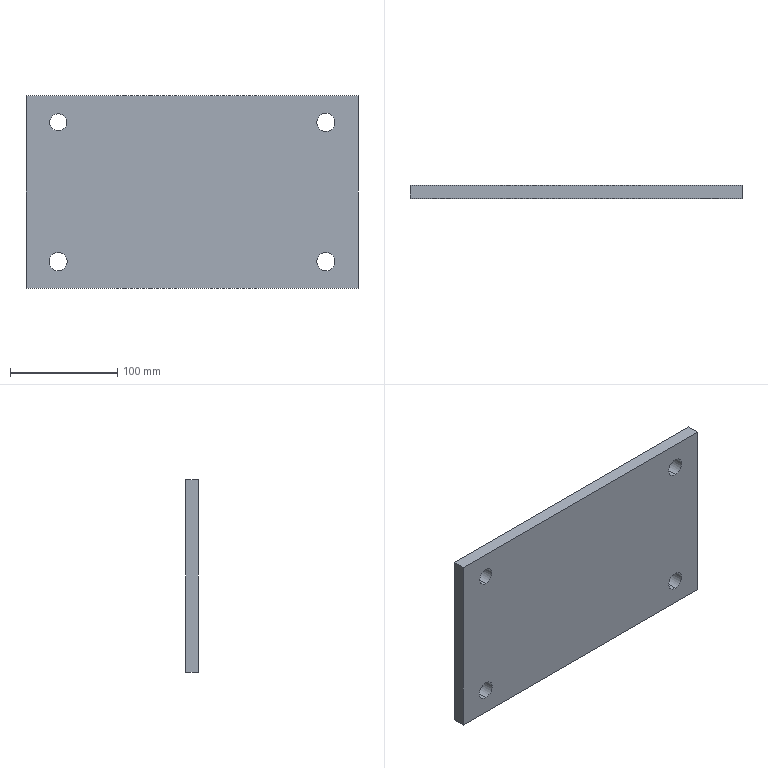Part | SolidWorks | features Extrusion 1 | 1 solid | 14 faces | box 310 x 12 x 180 mm | volume 659016 mm3 | cylinder 8 | plane 6 | commonest cylinder face diameters 17 x6 16 x2
STEP:
#1=CARTESIAN_POINT('',(125.,6.,-73.5));
#2=VERTEX_POINT('',#1);
#3=CARTESIAN_POINT('',(125.,6.,-56.5));
#4=VERTEX_POINT('',#3);
#5=CARTESIAN_POINT('',(125.,6.,-65.));
#6=DIRECTION('',(0.,1.,0.));
#7=DIRECTION('',(0.,0.,1.));
#8=AXIS2_PLACEMENT_3D('',#5,#6,#7);
#9=CIRCLE('',#8,8.5);
#10=EDGE_CURVE('',#2,#4,#9,.T.);
#11=ORIENTED_EDGE('',*,*,#10,.T.);
#12=CARTESIAN_POINT('',(125.,-6.,-56.5));
#13=VERTEX_POINT('',#12);
#14=CARTESIAN_POINT('',(125.,6.,-56.5));
#15=DIRECTION('',(0.,-1.,0.));
#16=VECTOR('',#15,1000.);
#17=LINE('',#14,#16);
#18=EDGE_CURVE('',#4,#13,#17,.T.);
#19=ORIENTED_EDGE('',*,*,#18,.T.);
#20=CARTESIAN_POINT('',(125.,-6.,-73.5));
#21=VERTEX_POINT('',#20);
#22=CARTESIAN_POINT('',(125.,-6.,-65.));
#23=DIRECTION('',(0.,1.,0.));
#24=DIRECTION('',(0.,0.,1.));
#25=AXIS2_PLACEMENT_3D('',#22,#23,#24);
#26=CIRCLE('',#25,8.5);
#27=EDGE_CURVE('',#21,#13,#26,.T.);
#28=ORIENTED_EDGE('',*,*,#27,.F.);
#29=CARTESIAN_POINT('',(125.,6.,-73.5));
#30=DIRECTION('',(0.,-1.,0.));
#31=VECTOR('',#30,1000.);
#32=LINE('',#29,#31);
#33=EDGE_CURVE('',#2,#21,#32,.T.);
#34=ORIENTED_EDGE('',*,*,#33,.F.);
#35=EDGE_LOOP('',(#11,#19,#28,#34));
#36=FACE_OUTER_BOUND('',#35,.T.);
#37=CARTESIAN_POINT('',(125.,6.,-65.));
#38=DIRECTION('',(0.,-1.,0.));
#39=DIRECTION('',(0.,0.,-1.));
#40=AXIS2_PLACEMENT_3D('',#37,#38,#39);
#41=CYLINDRICAL_SURFACE('',#40,8.5);
#42=ADVANCED_FACE('',(#36),#41,.F.);
#43=CARTESIAN_POINT('',(-125.,6.,-73.5));
#44=VERTEX_POINT('',#43);
#45=CARTESIAN_POINT('',(-125.,6.,-56.5));
#46=VERTEX_POINT('',#45);
#47=CARTESIAN_POINT('',(-125.,6.,-65.));
#48=DIRECTION('',(0.,1.,0.));
#49=DIRECTION('',(0.,0.,1.));
#50=AXIS2_PLACEMENT_3D('',#47,#48,#49);
#51=CIRCLE('',#50,8.5);
#52=EDGE_CURVE('',#44,#46,#51,.T.);
#53=ORIENTED_EDGE('',*,*,#52,.T.);
#54=CARTESIAN_POINT('',(-125.,-6.,-56.5));
#55=VERTEX_POINT('',#54);
#56=CARTESIAN_POINT('',(-125.,6.,-56.5));
#57=DIRECTION('',(0.,-1.,0.));
#58=VECTOR('',#57,1000.);
#59=LINE('',#56,#58);
#60=EDGE_CURVE('',#46,#55,#59,.T.);
#61=ORIENTED_EDGE('',*,*,#60,.T.);
#62=CARTESIAN_POINT('',(-125.,-6.,-73.5));
#63=VERTEX_POINT('',#62);
#64=CARTESIAN_POINT('',(-125.,-6.,-65.));
#65=DIRECTION('',(0.,1.,0.));
#66=DIRECTION('',(0.,0.,1.));
#67=AXIS2_PLACEMENT_3D('',#64,#65,#66);
#68=CIRCLE('',#67,8.5);
#69=EDGE_CURVE('',#63,#55,#68,.T.);
#70=ORIENTED_EDGE('',*,*,#69,.F.);
#71=CARTESIAN_POINT('',(-125.,6.,-73.5));
#72=DIRECTION('',(0.,-1.,0.));
#73=VECTOR('',#72,1000.);
#74=LINE('',#71,#73);
#75=EDGE_CURVE('',#44,#63,#74,.T.);
#76=ORIENTED_EDGE('',*,*,#75,.F.);
#77=EDGE_LOOP('',(#53,#61,#70,#76));
#78=FACE_OUTER_BOUND('',#77,.T.);
#79=CARTESIAN_POINT('',(-125.,6.,-65.));
#80=DIRECTION('',(0.,-1.,0.));
#81=DIRECTION('',(0.,0.,-1.));
#82=AXIS2_PLACEMENT_3D('',#79,#80,#81);
#83=CYLINDRICAL_SURFACE('',#82,8.5);
#84=ADVANCED_FACE('',(#78),#83,.F.);
#85=CARTESIAN_POINT('',(-125.,6.,57.));
#86=VERTEX_POINT('',#85);
#87=CARTESIAN_POINT('',(-125.,6.,73.));
#88=VERTEX_POINT('',#87);
#89=CARTESIAN_POINT('',(-125.,6.,65.));
#90=DIRECTION('',(0.,1.,0.));
#91=DIRECTION('',(0.,0.,1.));
#92=AXIS2_PLACEMENT_3D('',#89,#90,#91);
#93=CIRCLE('',#92,8.);
#94=EDGE_CURVE('',#86,#88,#93,.T.);
#95=ORIENTED_EDGE('',*,*,#94,.T.);
#96=CARTESIAN_POINT('',(-125.,-6.,73.));
#97=VERTEX_POINT('',#96);
#98=CARTESIAN_POINT('',(-125.,6.,73.));
#99=DIRECTION('',(0.,-1.,0.));
#100=VECTOR('',#99,1000.);
#101=LINE('',#98,#100);
#102=EDGE_CURVE('',#88,#97,#101,.T.);
#103=ORIENTED_EDGE('',*,*,#102,.T.);
#104=CARTESIAN_POINT('',(-125.,-6.,57.));
#105=VERTEX_POINT('',#104);
#106=CARTESIAN_POINT('',(-125.,-6.,65.));
#107=DIRECTION('',(0.,1.,0.));
#108=DIRECTION('',(0.,0.,1.));
#109=AXIS2_PLACEMENT_3D('',#106,#107,#108);
#110=CIRCLE('',#109,8.);
#111=EDGE_CURVE('',#105,#97,#110,.T.);
#112=ORIENTED_EDGE('',*,*,#111,.F.);
#113=CARTESIAN_POINT('',(-125.,6.,57.));
#114=DIRECTION('',(0.,-1.,0.));
#115=VECTOR('',#114,1000.);
#116=LINE('',#113,#115);
#117=EDGE_CURVE('',#86,#105,#116,.T.);
#118=ORIENTED_EDGE('',*,*,#117,.F.);
#119=EDGE_LOOP('',(#95,#103,#112,#118));
#120=FACE_OUTER_BOUND('',#119,.T.);
#121=CARTESIAN_POINT('',(-125.,6.,65.));
#122=DIRECTION('',(0.,-1.,0.));
#123=DIRECTION('',(0.,0.,-1.));
#124=AXIS2_PLACEMENT_3D('',#121,#122,#123);
#125=CYLINDRICAL_SURFACE('',#124,8.);
#126=ADVANCED_FACE('',(#120),#125,.F.);
#127=CARTESIAN_POINT('',(125.,6.,56.5));
#128=VERTEX_POINT('',#127);
#129=CARTESIAN_POINT('',(125.,6.,73.5));
#130=VERTEX_POINT('',#129);
#131=CARTESIAN_POINT('',(125.,6.,65.));
#132=DIRECTION('',(0.,1.,0.));
#133=DIRECTION('',(0.,0.,1.));
#134=AXIS2_PLACEMENT_3D('',#131,#132,#133);
#135=CIRCLE('',#134,8.5);
#136=EDGE_CURVE('',#128,#130,#135,.T.);
#137=ORIENTED_EDGE('',*,*,#136,.T.);
#138=CARTESIAN_POINT('',(125.,-6.,73.5));
#139=VERTEX_POINT('',#138);
#140=CARTESIAN_POINT('',(125.,6.,73.5));
#141=DIRECTION('',(0.,-1.,0.));
#142=VECTOR('',#141,1000.);
#143=LINE('',#140,#142);
#144=EDGE_CURVE('',#130,#139,#143,.T.);
#145=ORIENTED_EDGE('',*,*,#144,.T.);
#146=CARTESIAN_POINT('',(125.,-6.,56.5));
#147=VERTEX_POINT('',#146);
#148=CARTESIAN_POINT('',(125.,-6.,65.));
#149=DIRECTION('',(0.,1.,0.));
#150=DIRECTION('',(0.,0.,1.));
#151=AXIS2_PLACEMENT_3D('',#148,#149,#150);
#152=CIRCLE('',#151,8.5);
#153=EDGE_CURVE('',#147,#139,#152,.T.);
#154=ORIENTED_EDGE('',*,*,#153,.F.);
#155=CARTESIAN_POINT('',(125.,6.,56.5));
#156=DIRECTION('',(0.,-1.,0.));
#157=VECTOR('',#156,1000.);
#158=LINE('',#155,#157);
#159=EDGE_CURVE('',#128,#147,#158,.T.);
#160=ORIENTED_EDGE('',*,*,#159,.F.);
#161=EDGE_LOOP('',(#137,#145,#154,#160));
#162=FACE_OUTER_BOUND('',#161,.T.);
#163=CARTESIAN_POINT('',(125.,6.,65.));
#164=DIRECTION('',(0.,-1.,0.));
#165=DIRECTION('',(0.,0.,-1.));
#166=AXIS2_PLACEMENT_3D('',#163,#164,#165);
#167=CYLINDRICAL_SURFACE('',#166,8.5);
#168=ADVANCED_FACE('',(#162),#167,.F.);
#169=ORIENTED_EDGE('',*,*,#52,.F.);
#170=CARTESIAN_POINT('',(-125.,6.,-65.));
#171=DIRECTION('',(0.,1.,0.));
#172=DIRECTION('',(0.,0.,1.));
#173=AXIS2_PLACEMENT_3D('',#170,#171,#172);
#174=CIRCLE('',#173,8.5);
#175=EDGE_CURVE('',#46,#44,#174,.T.);
#176=ORIENTED_EDGE('',*,*,#175,.F.);
#177=EDGE_LOOP('',(#169,#176));
#178=FACE_BOUND('',#177,.T.);
#179=ORIENTED_EDGE('',*,*,#136,.F.);
#180=CARTESIAN_POINT('',(125.,6.,65.));
#181=DIRECTION('',(0.,1.,0.));
#182=DIRECTION('',(0.,0.,1.));
#183=AXIS2_PLACEMENT_3D('',#180,#181,#182);
#184=CIRCLE('',#183,8.5);
#185=EDGE_CURVE('',#130,#128,#184,.T.);
#186=ORIENTED_EDGE('',*,*,#185,.F.);
#187=EDGE_LOOP('',(#179,#186));
#188=FACE_BOUND('',#187,.T.);
#189=CARTESIAN_POINT('',(-155.,6.,-90.));
#190=VERTEX_POINT('',#189);
#191=CARTESIAN_POINT('',(-155.,6.,90.));
#192=VERTEX_POINT('',#191);
#193=CARTESIAN_POINT('',(-155.,6.,90.));
#194=DIRECTION('',(0.,0.,1.));
#195=VECTOR('',#194,1000.);
#196=LINE('',#193,#195);
#197=EDGE_CURVE('',#190,#192,#196,.T.);
#198=ORIENTED_EDGE('',*,*,#197,.T.);
#199=CARTESIAN_POINT('',(155.,6.,90.));
#200=VERTEX_POINT('',#199);
#201=CARTESIAN_POINT('',(155.,6.,90.));
#202=DIRECTION('',(1.,0.,0.));
#203=VECTOR('',#202,1000.);
#204=LINE('',#201,#203);
#205=EDGE_CURVE('',#192,#200,#204,.T.);
#206=ORIENTED_EDGE('',*,*,#205,.T.);
#207=CARTESIAN_POINT('',(155.,6.,-90.));
#208=VERTEX_POINT('',#207);
#209=CARTESIAN_POINT('',(155.,6.,-90.));
#210=DIRECTION('',(0.,0.,-1.));
#211=VECTOR('',#210,1000.);
#212=LINE('',#209,#211);
#213=EDGE_CURVE('',#200,#208,#212,.T.);
#214=ORIENTED_EDGE('',*,*,#213,.T.);
#215=CARTESIAN_POINT('',(-155.,6.,-90.));
#216=DIRECTION('',(-1.,0.,0.));
#217=VECTOR('',#216,1000.);
#218=LINE('',#215,#217);
#219=EDGE_CURVE('',#208,#190,#218,.T.);
#220=ORIENTED_EDGE('',*,*,#219,.T.);
#221=EDGE_LOOP('',(#198,#206,#214,#220));
#222=FACE_OUTER_BOUND('',#221,.T.);
#223=ORIENTED_EDGE('',*,*,#94,.F.);
#224=CARTESIAN_POINT('',(-125.,6.,65.));
#225=DIRECTION('',(0.,1.,0.));
#226=DIRECTION('',(0.,0.,1.));
#227=AXIS2_PLACEMENT_3D('',#224,#225,#226);
#228=CIRCLE('',#227,8.);
#229=EDGE_CURVE('',#88,#86,#228,.T.);
#230=ORIENTED_EDGE('',*,*,#229,.F.);
#231=EDGE_LOOP('',(#223,#230));
#232=FACE_BOUND('',#231,.T.);
#233=ORIENTED_EDGE('',*,*,#10,.F.);
#234=CARTESIAN_POINT('',(125.,6.,-65.));
#235=DIRECTION('',(0.,1.,0.));
#236=DIRECTION('',(0.,0.,1.));
#237=AXIS2_PLACEMENT_3D('',#234,#235,#236);
#238=CIRCLE('',#237,8.5);
#239=EDGE_CURVE('',#4,#2,#238,.T.);
#240=ORIENTED_EDGE('',*,*,#239,.F.);
#241=EDGE_LOOP('',(#233,#240));
#242=FACE_BOUND('',#241,.T.);
#243=CARTESIAN_POINT('',(-155.,6.,-90.));
#244=DIRECTION('',(0.,-1.,0.));
#245=DIRECTION('',(0.,0.,-1.));
#246=AXIS2_PLACEMENT_3D('',#243,#244,#245);
#247=PLANE('',#246);
#248=ADVANCED_FACE('',(#178,#188,#222,#232,#242),#247,.F.);
#249=ORIENTED_EDGE('',*,*,#69,.T.);
#250=CARTESIAN_POINT('',(-125.,-6.,-65.));
#251=DIRECTION('',(0.,1.,0.));
#252=DIRECTION('',(0.,0.,1.));
#253=AXIS2_PLACEMENT_3D('',#250,#251,#252);
#254=CIRCLE('',#253,8.5);
#255=EDGE_CURVE('',#55,#63,#254,.T.);
#256=ORIENTED_EDGE('',*,*,#255,.T.);
#257=EDGE_LOOP('',(#249,#256));
#258=FACE_BOUND('',#257,.T.);
#259=ORIENTED_EDGE('',*,*,#153,.T.);
#260=CARTESIAN_POINT('',(125.,-6.,65.));
#261=DIRECTION('',(0.,1.,0.));
#262=DIRECTION('',(0.,0.,1.));
#263=AXIS2_PLACEMENT_3D('',#260,#261,#262);
#264=CIRCLE('',#263,8.5);
#265=EDGE_CURVE('',#139,#147,#264,.T.);
#266=ORIENTED_EDGE('',*,*,#265,.T.);
#267=EDGE_LOOP('',(#259,#266));
#268=FACE_BOUND('',#267,.T.);
#269=CARTESIAN_POINT('',(-155.,-6.,-90.));
#270=VERTEX_POINT('',#269);
#271=CARTESIAN_POINT('',(-155.,-6.,90.));
#272=VERTEX_POINT('',#271);
#273=CARTESIAN_POINT('',(-155.,-6.,90.));
#274=DIRECTION('',(0.,0.,1.));
#275=VECTOR('',#274,1000.);
#276=LINE('',#273,#275);
#277=EDGE_CURVE('',#270,#272,#276,.T.);
#278=ORIENTED_EDGE('',*,*,#277,.F.);
#279=CARTESIAN_POINT('',(155.,-6.,-90.));
#280=VERTEX_POINT('',#279);
#281=CARTESIAN_POINT('',(-155.,-6.,-90.));
#282=DIRECTION('',(-1.,0.,0.));
#283=VECTOR('',#282,1000.);
#284=LINE('',#281,#283);
#285=EDGE_CURVE('',#280,#270,#284,.T.);
#286=ORIENTED_EDGE('',*,*,#285,.F.);
#287=CARTESIAN_POINT('',(155.,-6.,90.));
#288=VERTEX_POINT('',#287);
#289=CARTESIAN_POINT('',(155.,-6.,-90.));
#290=DIRECTION('',(0.,0.,-1.));
#291=VECTOR('',#290,1000.);
#292=LINE('',#289,#291);
#293=EDGE_CURVE('',#288,#280,#292,.T.);
#294=ORIENTED_EDGE('',*,*,#293,.F.);
#295=CARTESIAN_POINT('',(155.,-6.,90.));
#296=DIRECTION('',(1.,0.,0.));
#297=VECTOR('',#296,1000.);
#298=LINE('',#295,#297);
#299=EDGE_CURVE('',#272,#288,#298,.T.);
#300=ORIENTED_EDGE('',*,*,#299,.F.);
#301=EDGE_LOOP('',(#278,#286,#294,#300));
#302=FACE_OUTER_BOUND('',#301,.T.);
#303=ORIENTED_EDGE('',*,*,#111,.T.);
#304=CARTESIAN_POINT('',(-125.,-6.,65.));
#305=DIRECTION('',(0.,1.,0.));
#306=DIRECTION('',(0.,0.,1.));
#307=AXIS2_PLACEMENT_3D('',#304,#305,#306);
#308=CIRCLE('',#307,8.);
#309=EDGE_CURVE('',#97,#105,#308,.T.);
#310=ORIENTED_EDGE('',*,*,#309,.T.);
#311=EDGE_LOOP('',(#303,#310));
#312=FACE_BOUND('',#311,.T.);
#313=ORIENTED_EDGE('',*,*,#27,.T.);
#314=CARTESIAN_POINT('',(125.,-6.,-65.));
#315=DIRECTION('',(0.,1.,0.));
#316=DIRECTION('',(0.,0.,1.));
#317=AXIS2_PLACEMENT_3D('',#314,#315,#316);
#318=CIRCLE('',#317,8.5);
#319=EDGE_CURVE('',#13,#21,#318,.T.);
#320=ORIENTED_EDGE('',*,*,#319,.T.);
#321=EDGE_LOOP('',(#313,#320));
#322=FACE_BOUND('',#321,.T.);
#323=CARTESIAN_POINT('',(-155.,-6.,-90.));
#324=DIRECTION('',(0.,-1.,0.));
#325=DIRECTION('',(0.,0.,-1.));
#326=AXIS2_PLACEMENT_3D('',#323,#324,#325);
#327=PLANE('',#326);
#328=ADVANCED_FACE('',(#258,#268,#302,#312,#322),#327,.T.);
#329=ORIENTED_EDGE('',*,*,#277,.T.);
#330=CARTESIAN_POINT('',(-155.,6.,90.));
#331=DIRECTION('',(0.,-1.,0.));
#332=VECTOR('',#331,1000.);
#333=LINE('',#330,#332);
#334=EDGE_CURVE('',#192,#272,#333,.T.);
#335=ORIENTED_EDGE('',*,*,#334,.F.);
#336=ORIENTED_EDGE('',*,*,#197,.F.);
#337=CARTESIAN_POINT('',(-155.,6.,-90.));
#338=DIRECTION('',(0.,-1.,0.));
#339=VECTOR('',#338,1000.);
#340=LINE('',#337,#339);
#341=EDGE_CURVE('',#190,#270,#340,.T.);
#342=ORIENTED_EDGE('',*,*,#341,.T.);
#343=EDGE_LOOP('',(#329,#335,#336,#342));
#344=FACE_OUTER_BOUND('',#343,.T.);
#345=CARTESIAN_POINT('',(-155.,6.,90.));
#346=DIRECTION('',(1.,0.,0.));
#347=DIRECTION('',(0.,0.,-1.));
#348=AXIS2_PLACEMENT_3D('',#345,#346,#347);
#349=PLANE('',#348);
#350=ADVANCED_FACE('',(#344),#349,.F.);
#351=ORIENTED_EDGE('',*,*,#299,.T.);
#352=CARTESIAN_POINT('',(155.,6.,90.));
#353=DIRECTION('',(0.,-1.,0.));
#354=VECTOR('',#353,1000.);
#355=LINE('',#352,#354);
#356=EDGE_CURVE('',#200,#288,#355,.T.);
#357=ORIENTED_EDGE('',*,*,#356,.F.);
#358=ORIENTED_EDGE('',*,*,#205,.F.);
#359=ORIENTED_EDGE('',*,*,#334,.T.);
#360=EDGE_LOOP('',(#351,#357,#358,#359));
#361=FACE_OUTER_BOUND('',#360,.T.);
#362=CARTESIAN_POINT('',(155.,6.,90.));
#363=DIRECTION('',(0.,0.,-1.));
#364=DIRECTION('',(-1.,0.,0.));
#365=AXIS2_PLACEMENT_3D('',#362,#363,#364);
#366=PLANE('',#365);
#367=ADVANCED_FACE('',(#361),#366,.F.);
#368=ORIENTED_EDGE('',*,*,#293,.T.);
#369=CARTESIAN_POINT('',(155.,6.,-90.));
#370=DIRECTION('',(0.,-1.,0.));
#371=VECTOR('',#370,1000.);
#372=LINE('',#369,#371);
#373=EDGE_CURVE('',#208,#280,#372,.T.);
#374=ORIENTED_EDGE('',*,*,#373,.F.);
#375=ORIENTED_EDGE('',*,*,#213,.F.);
#376=ORIENTED_EDGE('',*,*,#356,.T.);
#377=EDGE_LOOP('',(#368,#374,#375,#376));
#378=FACE_OUTER_BOUND('',#377,.T.);
#379=CARTESIAN_POINT('',(155.,6.,-90.));
#380=DIRECTION('',(-1.,0.,0.));
#381=DIRECTION('',(0.,0.,1.));
#382=AXIS2_PLACEMENT_3D('',#379,#380,#381);
#383=PLANE('',#382);
#384=ADVANCED_FACE('',(#378),#383,.F.);
#385=ORIENTED_EDGE('',*,*,#285,.T.);
#386=ORIENTED_EDGE('',*,*,#341,.F.);
#387=ORIENTED_EDGE('',*,*,#219,.F.);
#388=ORIENTED_EDGE('',*,*,#373,.T.);
#389=EDGE_LOOP('',(#385,#386,#387,#388));
#390=FACE_OUTER_BOUND('',#389,.T.);
#391=CARTESIAN_POINT('',(-155.,6.,-90.));
#392=DIRECTION('',(0.,0.,1.));
#393=DIRECTION('',(1.,0.,0.));
#394=AXIS2_PLACEMENT_3D('',#391,#392,#393);
#395=PLANE('',#394);
#396=ADVANCED_FACE('',(#390),#395,.F.);
#397=ORIENTED_EDGE('',*,*,#144,.F.);
#398=ORIENTED_EDGE('',*,*,#185,.T.);
#399=ORIENTED_EDGE('',*,*,#159,.T.);
#400=ORIENTED_EDGE('',*,*,#265,.F.);
#401=EDGE_LOOP('',(#397,#398,#399,#400));
#402=FACE_OUTER_BOUND('',#401,.T.);
#403=CARTESIAN_POINT('',(125.,6.,65.));
#404=DIRECTION('',(0.,-1.,0.));
#405=DIRECTION('',(0.,0.,-1.));
#406=AXIS2_PLACEMENT_3D('',#403,#404,#405);
#407=CYLINDRICAL_SURFACE('',#406,8.5);
#408=ADVANCED_FACE('',(#402),#407,.F.);
#409=ORIENTED_EDGE('',*,*,#102,.F.);
#410=ORIENTED_EDGE('',*,*,#229,.T.);
#411=ORIENTED_EDGE('',*,*,#117,.T.);
#412=ORIENTED_EDGE('',*,*,#309,.F.);
#413=EDGE_LOOP('',(#409,#410,#411,#412));
#414=FACE_OUTER_BOUND('',#413,.T.);
#415=CARTESIAN_POINT('',(-125.,6.,65.));
#416=DIRECTION('',(0.,-1.,0.));
#417=DIRECTION('',(0.,0.,-1.));
#418=AXIS2_PLACEMENT_3D('',#415,#416,#417);
#419=CYLINDRICAL_SURFACE('',#418,8.);
#420=ADVANCED_FACE('',(#414),#419,.F.);
#421=ORIENTED_EDGE('',*,*,#60,.F.);
#422=ORIENTED_EDGE('',*,*,#175,.T.);
#423=ORIENTED_EDGE('',*,*,#75,.T.);
#424=ORIENTED_EDGE('',*,*,#255,.F.);
#425=EDGE_LOOP('',(#421,#422,#423,#424));
#426=FACE_OUTER_BOUND('',#425,.T.);
#427=CARTESIAN_POINT('',(-125.,6.,-65.));
#428=DIRECTION('',(0.,-1.,0.));
#429=DIRECTION('',(0.,0.,-1.));
#430=AXIS2_PLACEMENT_3D('',#427,#428,#429);
#431=CYLINDRICAL_SURFACE('',#430,8.5);
#432=ADVANCED_FACE('',(#426),#431,.F.);
#433=ORIENTED_EDGE('',*,*,#18,.F.);
#434=ORIENTED_EDGE('',*,*,#239,.T.);
#435=ORIENTED_EDGE('',*,*,#33,.T.);
#436=ORIENTED_EDGE('',*,*,#319,.F.);
#437=EDGE_LOOP('',(#433,#434,#435,#436));
#438=FACE_OUTER_BOUND('',#437,.T.);
#439=CARTESIAN_POINT('',(125.,6.,-65.));
#440=DIRECTION('',(0.,-1.,0.));
#441=DIRECTION('',(0.,0.,-1.));
#442=AXIS2_PLACEMENT_3D('',#439,#440,#441);
#443=CYLINDRICAL_SURFACE('',#442,8.5);
#444=ADVANCED_FACE('',(#438),#443,.F.);
#445=CLOSED_SHELL('',(#42,#84,#126,#168,#248,#328,#350,#367,#384,#396,#408,#420,#432,#444));
#446=MANIFOLD_SOLID_BREP('',#445);
#447=CARTESIAN_POINT('',(0.,0.,0.));
#448=DIRECTION('',(0.,0.,1.));
#449=DIRECTION('',(1.,0.,0.));
#450=AXIS2_PLACEMENT_3D('',#447,#448,#449);
#451=(LENGTH_UNIT()NAMED_UNIT(*)SI_UNIT(.MILLI.,.METRE.));
#452=UNCERTAINTY_MEASURE_WITH_UNIT(LENGTH_MEASURE(0.00001),#451,'','');
#453=(NAMED_UNIT(*)PLANE_ANGLE_UNIT()SI_UNIT($,.RADIAN.));
#454=(NAMED_UNIT(*)SI_UNIT($,.STERADIAN.)SOLID_ANGLE_UNIT());
#455=(GEOMETRIC_REPRESENTATION_CONTEXT(3)GLOBAL_UNCERTAINTY_ASSIGNED_CONTEXT((#452))GLOBAL_UNIT_ASSIGNED_CONTEXT((#451,#453,#454))REPRESENTATION_CONTEXT('',''));
#456=ADVANCED_BREP_SHAPE_REPRESENTATION('',(#446,#450),#455);